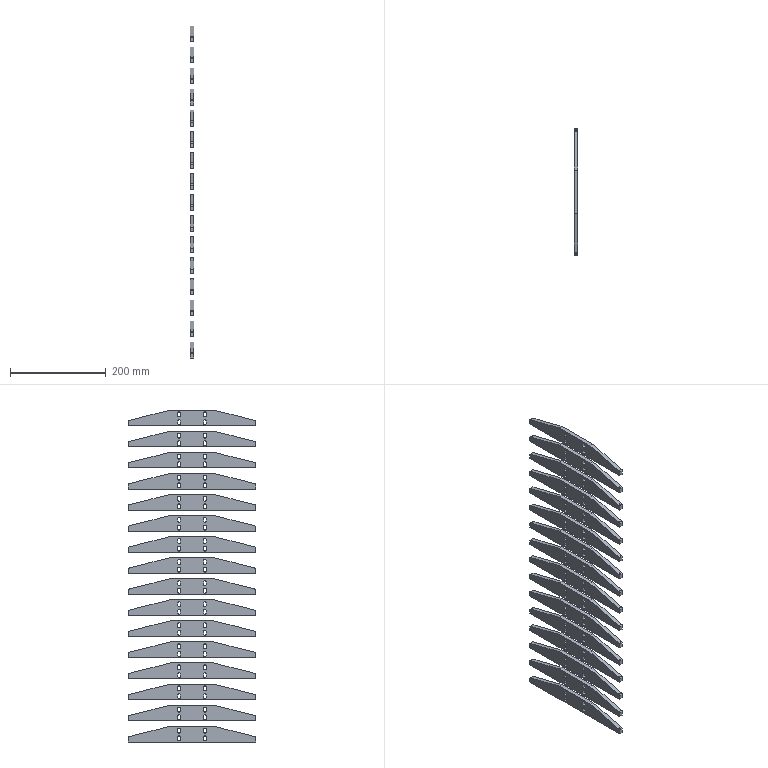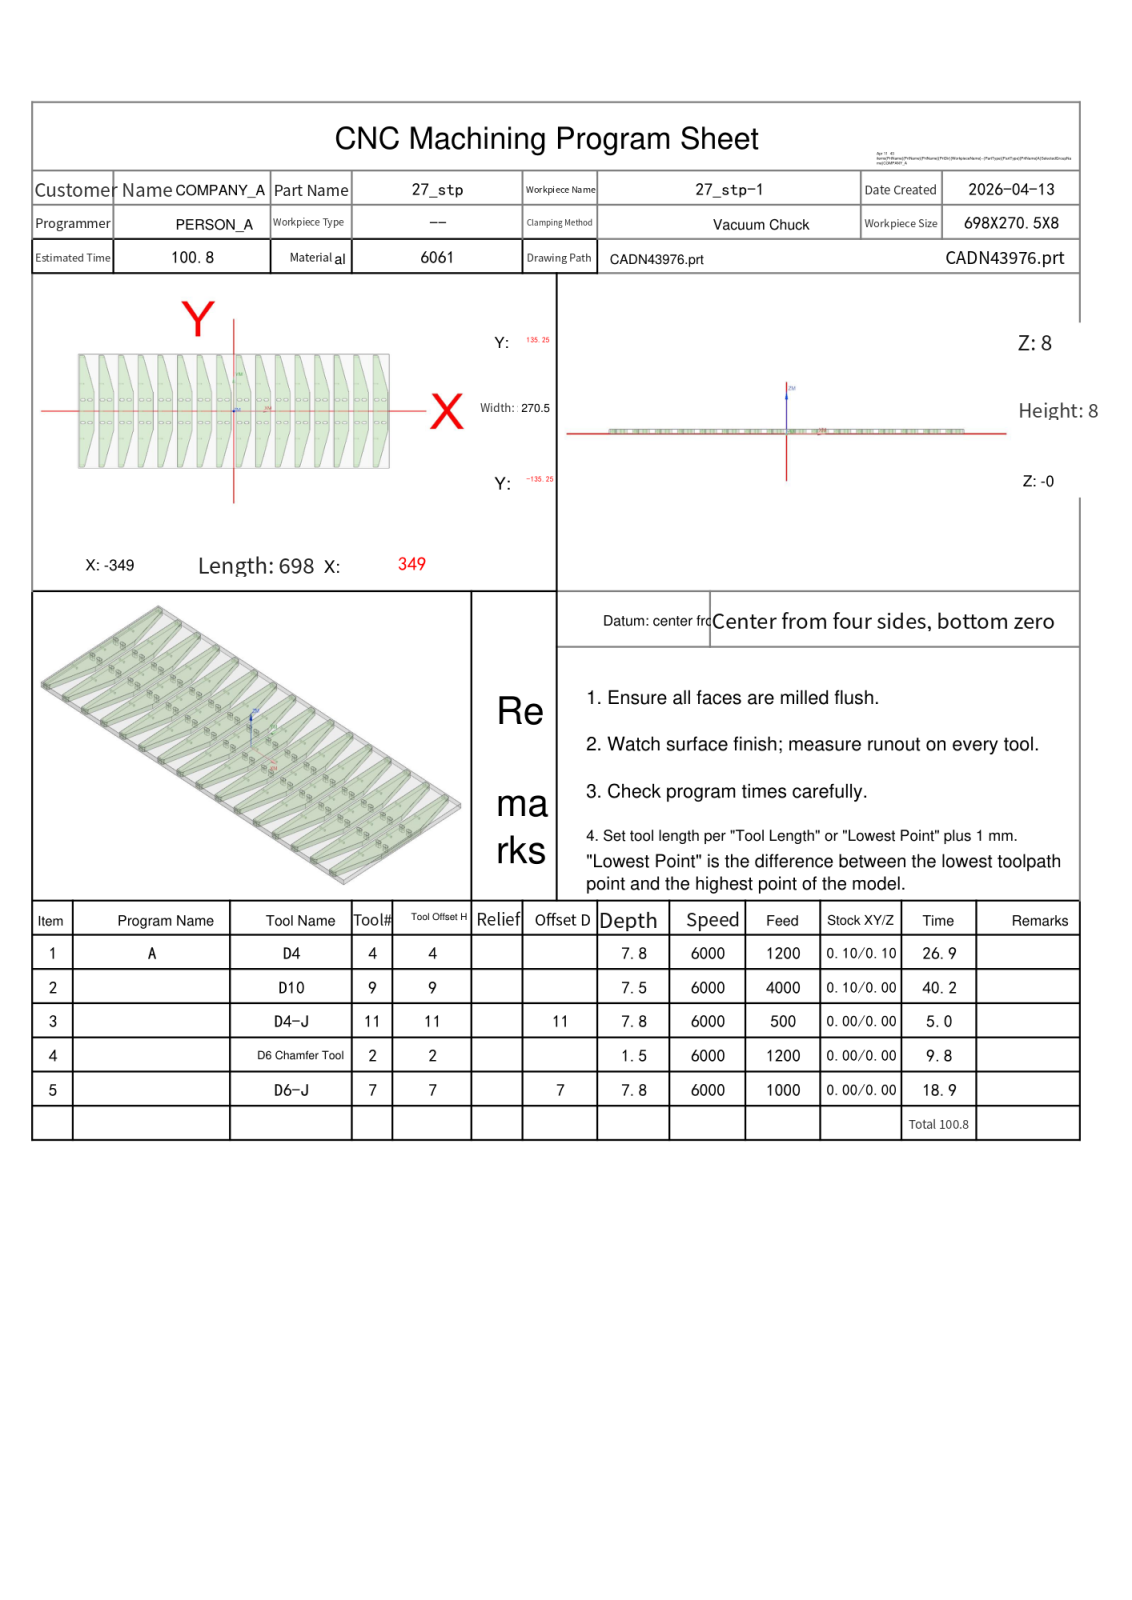NC program | NX | posted by the shop | part box 8 x 265.5 x 693 mm
Lines 19372 to 21683 of 21683, first 1858 of 2312 lines:
N4 T02 M06
(D6 Chamfer Tool  D=6. R=0. H=02 ce=0.00 di=0.00)
G00 G90 G54 X311.372 Y-.25 M03 S6000
G43 H02 Z28.
M08
Z10.099
G01 Z6.5 F1200.
G03 X311.672 Y-.33 I.3 J.52
X312.192 Y-.03 I0.0 J.6
G01 X312.2 Y0.0
Y132.75
G02 X313.5 Y134.05 I1.3 J0.0
G01 X322.012
G02 X326.18 Y130.804 I0.0 J-4.3
G01 X347.76 Y45.484
X347.79 Y45.326
X347.8 Y45.166
Y-45.166
X347.79 Y-45.326
X347.76 Y-45.484
X326.18 Y-130.804
G02 X322.012 Y-134.05 I-4.169 J1.054
G01 X313.5
G02 X312.2 Y-132.75 I0.0 J1.3
G01 Y0.0
X312.192 Y.03
G03 X311.672 Y.33 I-.52 J-.3
X311.372 Y.25 I0.0 J-.6
G01 Z10.099
G00 Z28.
X336.95 Y26.378
Z10.099
G01 Z6.5
G03 X336.87 Y26.078 I.52 J-.3
X337.17 Y25.558 I.6 J0.0
G01 X337.2 Y25.55
X339.7
G03 X341.15 Y27. I0.0 J1.45
X339.7 Y28.45 I-1.45 J0.0
G01 X334.7
G03 X333.25 Y27. I0.0 J-1.45
X334.7 Y25.55 I1.45 J0.0
G01 X337.2
X337.23 Y25.558
G03 X337.53 Y26.078 I-.3 J.52
X337.45 Y26.378 I-.6 J0.0
G01 Z10.099
G00 Z28.
X320.95
Z10.099
G01 Z6.5
G03 X320.87 Y26.078 I.52 J-.3
X321.17 Y25.558 I.6 J0.0
G01 X321.2 Y25.55
X323.7
G03 X325.15 Y27. I0.0 J1.45
X323.7 Y28.45 I-1.45 J0.0
G01 X318.7
G03 X317.25 Y27. I0.0 J-1.45
X318.7 Y25.55 I1.45 J0.0
G01 X321.2
X321.23 Y25.558
G03 X321.53 Y26.078 I-.3 J.52
X321.45 Y26.378 I-.6 J0.0
G01 Z10.099
G00 Z28.
X320.95 Y-27.622
Z10.099
G01 Z6.5
G03 X320.87 Y-27.922 I.52 J-.3
X321.17 Y-28.442 I.6 J0.0
G01 X321.2 Y-28.45
X323.7
G03 X325.15 Y-27. I0.0 J1.45
X323.7 Y-25.55 I-1.45 J0.0
G01 X318.7
G03 X317.25 Y-27. I0.0 J-1.45
X318.7 Y-28.45 I1.45 J0.0
G01 X321.2
X321.23 Y-28.442
G03 X321.53 Y-27.922 I-.3 J.52
X321.45 Y-27.622 I-.6 J0.0
G01 Z10.099
G00 Z28.
X336.95
Z10.099
G01 Z6.5
G03 X336.87 Y-27.922 I.52 J-.3
X337.17 Y-28.442 I.6 J0.0
G01 X337.2 Y-28.45
X339.7
G03 X341.15 Y-27. I0.0 J1.45
X339.7 Y-25.55 I-1.45 J0.0
G01 X334.7
G03 X333.25 Y-27. I0.0 J-1.45
X334.7 Y-28.45 I1.45 J0.0
G01 X337.2
X337.23 Y-28.442
G03 X337.53 Y-27.922 I-.3 J.52
X337.45 Y-27.622 I-.6 J0.0
G01 Z10.099
G00 Z28.
X267.372 Y-.25
Z10.099
G01 Z6.5
G03 X267.672 Y-.33 I.3 J.52
X268.192 Y-.03 I0.0 J.6
G01 X268.2 Y0.0
Y132.75
G02 X269.5 Y134.05 I1.3 J0.0
G01 X278.012
G02 X282.18 Y130.804 I0.0 J-4.3
G01 X303.76 Y45.484
X303.79 Y45.326
X303.8 Y45.166
Y-45.166
X303.79 Y-45.326
X303.76 Y-45.484
X282.18 Y-130.804
G02 X278.012 Y-134.05 I-4.169 J1.054
G01 X269.5
G02 X268.2 Y-132.75 I0.0 J1.3
G01 Y0.0
X268.192 Y.03
G03 X267.672 Y.33 I-.52 J-.3
X267.372 Y.25 I0.0 J-.6
G01 Z10.099
G00 Z28.
X293.45 Y27.622
Z10.099
G01 Z6.5
G03 X293.53 Y27.922 I-.52 J.3
X293.23 Y28.442 I-.6 J0.0
G01 X293.2 Y28.45
X290.7
G03 X289.25 Y27. I0.0 J-1.45
X290.7 Y25.55 I1.45 J0.0
G01 X295.7
G03 X297.15 Y27. I0.0 J1.45
X295.7 Y28.45 I-1.45 J0.0
G01 X293.2
X293.17 Y28.442
G03 X292.87 Y27.922 I.3 J-.52
X292.95 Y27.622 I.6 J0.0
G01 Z10.099
G00 Z28.
X277.45
Z10.099
G01 Z6.5
G03 X277.53 Y27.922 I-.52 J.3
X277.23 Y28.442 I-.6 J0.0
G01 X277.2 Y28.45
X274.7
G03 X273.25 Y27. I0.0 J-1.45
X274.7 Y25.55 I1.45 J0.0
G01 X279.7
G03 X281.15 Y27. I0.0 J1.45
X279.7 Y28.45 I-1.45 J0.0
G01 X277.2
X277.17 Y28.442
G03 X276.87 Y27.922 I.3 J-.52
X276.95 Y27.622 I.6 J0.0
G01 Z10.099
G00 Z28.
X277.45 Y-26.378
Z10.099
G01 Z6.5
G03 X277.53 Y-26.078 I-.52 J.3
X277.23 Y-25.558 I-.6 J0.0
G01 X277.2 Y-25.55
X274.7
G03 X273.25 Y-27. I0.0 J-1.45
X274.7 Y-28.45 I1.45 J0.0
G01 X279.7
G03 X281.15 Y-27. I0.0 J1.45
X279.7 Y-25.55 I-1.45 J0.0
G01 X277.2
X277.17 Y-25.558
G03 X276.87 Y-26.078 I.3 J-.52
X276.95 Y-26.378 I.6 J0.0
G01 Z10.099
G00 Z28.
X292.95 Y-27.622
Z10.099
G01 Z6.5
G03 X292.87 Y-27.922 I.52 J-.3
X293.17 Y-28.442 I.6 J0.0
G01 X293.2 Y-28.45
X295.7
G03 X297.15 Y-27. I0.0 J1.45
X295.7 Y-25.55 I-1.45 J0.0
G01 X290.7
G03 X289.25 Y-27. I0.0 J-1.45
X290.7 Y-28.45 I1.45 J0.0
G01 X293.2
X293.23 Y-28.442
G03 X293.53 Y-27.922 I-.3 J.52
X293.45 Y-27.622 I-.6 J0.0
G01 Z10.099
G00 Z28.
X223.372 Y-.25
Z10.099
G01 Z6.5
G03 X223.672 Y-.33 I.3 J.52
X224.192 Y-.03 I0.0 J.6
G01 X224.2 Y0.0
Y132.75
G02 X225.5 Y134.05 I1.3 J0.0
G01 X234.012
G02 X238.18 Y130.804 I0.0 J-4.3
G01 X259.76 Y45.484
X259.79 Y45.326
X259.8 Y45.166
Y-45.166
X259.79 Y-45.326
X259.76 Y-45.484
X238.18 Y-130.804
G02 X234.012 Y-134.05 I-4.169 J1.054
G01 X225.5
G02 X224.2 Y-132.75 I0.0 J1.3
G01 Y0.0
X224.192 Y.03
G03 X223.672 Y.33 I-.52 J-.3
X223.372 Y.25 I0.0 J-.6
G01 Z10.099
G00 Z28.
X248.95 Y26.378
Z10.099
G01 Z6.5
G03 X248.87 Y26.078 I.52 J-.3
X249.17 Y25.558 I.6 J0.0
G01 X249.2 Y25.55
X251.7
G03 X253.15 Y27. I0.0 J1.45
X251.7 Y28.45 I-1.45 J0.0
G01 X246.7
G03 X245.25 Y27. I0.0 J-1.45
X246.7 Y25.55 I1.45 J0.0
G01 X249.2
X249.23 Y25.558
G03 X249.53 Y26.078 I-.3 J.52
X249.45 Y26.378 I-.6 J0.0
G01 Z10.099
G00 Z28.
X232.95
Z10.099
G01 Z6.5
G03 X232.87 Y26.078 I.52 J-.3
X233.17 Y25.558 I.6 J0.0
G01 X233.2 Y25.55
X235.7
G03 X237.15 Y27. I0.0 J1.45
X235.7 Y28.45 I-1.45 J0.0
G01 X230.7
G03 X229.25 Y27. I0.0 J-1.45
X230.7 Y25.55 I1.45 J0.0
G01 X233.2
X233.23 Y25.558
G03 X233.53 Y26.078 I-.3 J.52
X233.45 Y26.378 I-.6 J0.0
G01 Z10.099
G00 Z28.
Y-26.378
Z10.099
G01 Z6.5
G03 X233.53 Y-26.078 I-.52 J.3
X233.23 Y-25.558 I-.6 J0.0
G01 X233.2 Y-25.55
X230.7
G03 X229.25 Y-27. I0.0 J-1.45
X230.7 Y-28.45 I1.45 J0.0
G01 X235.7
G03 X237.15 Y-27. I0.0 J1.45
X235.7 Y-25.55 I-1.45 J0.0
G01 X233.2
X233.17 Y-25.558
G03 X232.87 Y-26.078 I.3 J-.52
X232.95 Y-26.378 I.6 J0.0
G01 Z10.099
G00 Z28.
X249.45
Z10.099
G01 Z6.5
G03 X249.53 Y-26.078 I-.52 J.3
X249.23 Y-25.558 I-.6 J0.0
G01 X249.2 Y-25.55
X246.7
G03 X245.25 Y-27. I0.0 J-1.45
X246.7 Y-28.45 I1.45 J0.0
G01 X251.7
G03 X253.15 Y-27. I0.0 J1.45
X251.7 Y-25.55 I-1.45 J0.0
G01 X249.2
X249.17 Y-25.558
G03 X248.87 Y-26.078 I.3 J-.52
X248.95 Y-26.378 I.6 J0.0
G01 Z10.099
G00 Z28.
X179.372 Y-.25
Z10.099
G01 Z6.5
G03 X179.672 Y-.33 I.3 J.52
X180.192 Y-.03 I0.0 J.6
G01 X180.2 Y0.0
Y132.75
G02 X181.5 Y134.05 I1.3 J0.0
G01 X190.012
G02 X194.18 Y130.804 I0.0 J-4.3
G01 X215.76 Y45.484
X215.79 Y45.326
X215.8 Y45.166
Y-45.166
X215.79 Y-45.326
X215.76 Y-45.484
X194.18 Y-130.804
G02 X190.012 Y-134.05 I-4.169 J1.054
G01 X181.5
G02 X180.2 Y-132.75 I0.0 J1.3
G01 Y0.0
X180.192 Y.03
G03 X179.672 Y.33 I-.52 J-.3
X179.372 Y.25 I0.0 J-.6
G01 Z10.099
G00 Z28.
X204.95 Y26.378
Z10.099
G01 Z6.5
G03 X204.87 Y26.078 I.52 J-.3
X205.17 Y25.558 I.6 J0.0
G01 X205.2 Y25.55
X207.7
G03 X209.15 Y27. I0.0 J1.45
X207.7 Y28.45 I-1.45 J0.0
G01 X202.7
G03 X201.25 Y27. I0.0 J-1.45
X202.7 Y25.55 I1.45 J0.0
G01 X205.2
X205.23 Y25.558
G03 X205.53 Y26.078 I-.3 J.52
X205.45 Y26.378 I-.6 J0.0
G01 Z10.099
G00 Z28.
X188.95
Z10.099
G01 Z6.5
G03 X188.87 Y26.078 I.52 J-.3
X189.17 Y25.558 I.6 J0.0
G01 X189.2 Y25.55
X191.7
G03 X193.15 Y27. I0.0 J1.45
X191.7 Y28.45 I-1.45 J0.0
G01 X186.7
G03 X185.25 Y27. I0.0 J-1.45
X186.7 Y25.55 I1.45 J0.0
G01 X189.2
X189.23 Y25.558
G03 X189.53 Y26.078 I-.3 J.52
X189.45 Y26.378 I-.6 J0.0
G01 Z10.099
G00 Z28.
Y-26.378
Z10.099
G01 Z6.5
G03 X189.53 Y-26.078 I-.52 J.3
X189.23 Y-25.558 I-.6 J0.0
G01 X189.2 Y-25.55
X186.7
G03 X185.25 Y-27. I0.0 J-1.45
X186.7 Y-28.45 I1.45 J0.0
G01 X191.7
G03 X193.15 Y-27. I0.0 J1.45
X191.7 Y-25.55 I-1.45 J0.0
G01 X189.2
X189.17 Y-25.558
G03 X188.87 Y-26.078 I.3 J-.52
X188.95 Y-26.378 I.6 J0.0
G01 Z10.099
G00 Z28.
X205.45
Z10.099
G01 Z6.5
G03 X205.53 Y-26.078 I-.52 J.3
X205.23 Y-25.558 I-.6 J0.0
G01 X205.2 Y-25.55
X202.7
G03 X201.25 Y-27. I0.0 J-1.45
X202.7 Y-28.45 I1.45 J0.0
G01 X207.7
G03 X209.15 Y-27. I0.0 J1.45
X207.7 Y-25.55 I-1.45 J0.0
G01 X205.2
X205.17 Y-25.558
G03 X204.87 Y-26.078 I.3 J-.52
X204.95 Y-26.378 I.6 J0.0
G01 Z10.099
G00 Z28.
X135.372 Y-.25
Z10.099
G01 Z6.5
G03 X135.672 Y-.33 I.3 J.52
X136.192 Y-.03 I0.0 J.6
G01 X136.2 Y0.0
Y132.75
G02 X137.5 Y134.05 I1.3 J0.0
G01 X146.012
G02 X150.18 Y130.804 I0.0 J-4.3
G01 X171.76 Y45.484
X171.79 Y45.326
X171.8 Y45.166
Y-45.166
X171.79 Y-45.326
X171.76 Y-45.484
X150.18 Y-130.804
G02 X146.012 Y-134.05 I-4.169 J1.054
G01 X137.5
G02 X136.2 Y-132.75 I0.0 J1.3
G01 Y0.0
X136.192 Y.03
G03 X135.672 Y.33 I-.52 J-.3
X135.372 Y.25 I0.0 J-.6
G01 Z10.099
G00 Z28.
X160.95 Y26.378
Z10.099
G01 Z6.5
G03 X160.87 Y26.078 I.52 J-.3
X161.17 Y25.558 I.6 J0.0
G01 X161.2 Y25.55
X163.7
G03 X165.15 Y27. I0.0 J1.45
X163.7 Y28.45 I-1.45 J0.0
G01 X158.7
G03 X157.25 Y27. I0.0 J-1.45
X158.7 Y25.55 I1.45 J0.0
G01 X161.2
X161.23 Y25.558
G03 X161.53 Y26.078 I-.3 J.52
X161.45 Y26.378 I-.6 J0.0
G01 Z10.099
G00 Z28.
X144.95
Z10.099
G01 Z6.5
G03 X144.87 Y26.078 I.52 J-.3
X145.17 Y25.558 I.6 J0.0
G01 X145.2 Y25.55
X147.7
G03 X149.15 Y27. I0.0 J1.45
X147.7 Y28.45 I-1.45 J0.0
G01 X142.7
G03 X141.25 Y27. I0.0 J-1.45
X142.7 Y25.55 I1.45 J0.0
G01 X145.2
X145.23 Y25.558
G03 X145.53 Y26.078 I-.3 J.52
X145.45 Y26.378 I-.6 J0.0
G01 Z10.099
G00 Z28.
Y-26.378
Z10.099
G01 Z6.5
G03 X145.53 Y-26.078 I-.52 J.3
X145.23 Y-25.558 I-.6 J0.0
G01 X145.2 Y-25.55
X142.7
G03 X141.25 Y-27. I0.0 J-1.45
X142.7 Y-28.45 I1.45 J0.0
G01 X147.7
G03 X149.15 Y-27. I0.0 J1.45
X147.7 Y-25.55 I-1.45 J0.0
G01 X145.2
X145.17 Y-25.558
G03 X144.87 Y-26.078 I.3 J-.52
X144.95 Y-26.378 I.6 J0.0
G01 Z10.099
G00 Z28.
X161.45
Z10.099
G01 Z6.5
G03 X161.53 Y-26.078 I-.52 J.3
X161.23 Y-25.558 I-.6 J0.0
G01 X161.2 Y-25.55
X158.7
G03 X157.25 Y-27. I0.0 J-1.45
X158.7 Y-28.45 I1.45 J0.0
G01 X163.7
G03 X165.15 Y-27. I0.0 J1.45
X163.7 Y-25.55 I-1.45 J0.0
G01 X161.2
X161.17 Y-25.558
G03 X160.87 Y-26.078 I.3 J-.52
X160.95 Y-26.378 I.6 J0.0
G01 Z10.099
G00 Z28.
X91.372 Y-.25
Z10.099
G01 Z6.5
G03 X91.672 Y-.33 I.3 J.52
X92.192 Y-.03 I0.0 J.6
G01 X92.2 Y0.0
Y132.75
G02 X93.5 Y134.05 I1.3 J0.0
G01 X102.012
G02 X106.18 Y130.804 I0.0 J-4.3
G01 X127.76 Y45.484
X127.79 Y45.326
X127.8 Y45.166
Y-45.166
X127.79 Y-45.326
X127.76 Y-45.484
X106.18 Y-130.804
G02 X102.012 Y-134.05 I-4.169 J1.054
G01 X93.5
G02 X92.2 Y-132.75 I0.0 J1.3
G01 Y0.0
X92.192 Y.03
G03 X91.672 Y.33 I-.52 J-.3
X91.372 Y.25 I0.0 J-.6
G01 Z10.099
G00 Z28.
X116.95 Y26.378
Z10.099
G01 Z6.5
G03 X116.87 Y26.078 I.52 J-.3
X117.17 Y25.558 I.6 J0.0
G01 X117.2 Y25.55
X119.7
G03 X121.15 Y27. I0.0 J1.45
X119.7 Y28.45 I-1.45 J0.0
G01 X114.7
G03 X113.25 Y27. I0.0 J-1.45
X114.7 Y25.55 I1.45 J0.0
G01 X117.2
X117.23 Y25.558
G03 X117.53 Y26.078 I-.3 J.52
X117.45 Y26.378 I-.6 J0.0
G01 Z10.099
G00 Z28.
X100.95
Z10.099
G01 Z6.5
G03 X100.87 Y26.078 I.52 J-.3
X101.17 Y25.558 I.6 J0.0
G01 X101.2 Y25.55
X103.7
G03 X105.15 Y27. I0.0 J1.45
X103.7 Y28.45 I-1.45 J0.0
G01 X98.7
G03 X97.25 Y27. I0.0 J-1.45
X98.7 Y25.55 I1.45 J0.0
G01 X101.2
X101.23 Y25.558
G03 X101.53 Y26.078 I-.3 J.52
X101.45 Y26.378 I-.6 J0.0
G01 Z10.099
G00 Z28.
Y-26.378
Z10.099
G01 Z6.5
G03 X101.53 Y-26.078 I-.52 J.3
X101.23 Y-25.558 I-.6 J0.0
G01 X101.2 Y-25.55
X98.7
G03 X97.25 Y-27. I0.0 J-1.45
X98.7 Y-28.45 I1.45 J0.0
G01 X103.7
G03 X105.15 Y-27. I0.0 J1.45
X103.7 Y-25.55 I-1.45 J0.0
G01 X101.2
X101.17 Y-25.558
G03 X100.87 Y-26.078 I.3 J-.52
X100.95 Y-26.378 I.6 J0.0
G01 Z10.099
G00 Z28.
X117.45
Z10.099
G01 Z6.5
G03 X117.53 Y-26.078 I-.52 J.3
X117.23 Y-25.558 I-.6 J0.0
G01 X117.2 Y-25.55
X114.7
G03 X113.25 Y-27. I0.0 J-1.45
X114.7 Y-28.45 I1.45 J0.0
G01 X119.7
G03 X121.15 Y-27. I0.0 J1.45
X119.7 Y-25.55 I-1.45 J0.0
G01 X117.2
X117.17 Y-25.558
G03 X116.87 Y-26.078 I.3 J-.52
X116.95 Y-26.378 I.6 J0.0
G01 Z10.099
G00 Z28.
X47.372 Y-.25
Z10.099
G01 Z6.5
G03 X47.672 Y-.33 I.3 J.52
X48.192 Y-.03 I0.0 J.6
G01 X48.2 Y0.0
Y132.75
G02 X49.5 Y134.05 I1.3 J0.0
G01 X58.012
G02 X62.18 Y130.804 I0.0 J-4.3
G01 X83.76 Y45.484
X83.79 Y45.326
X83.8 Y45.166
Y-45.166
X83.79 Y-45.326
X83.76 Y-45.484
X62.18 Y-130.804
G02 X58.012 Y-134.05 I-4.169 J1.054
G01 X49.5
G02 X48.2 Y-132.75 I0.0 J1.3
G01 Y0.0
X48.192 Y.03
G03 X47.672 Y.33 I-.52 J-.3
X47.372 Y.25 I0.0 J-.6
G01 Z10.099
G00 Z28.
X72.95 Y26.378
Z10.099
G01 Z6.5
G03 X72.87 Y26.078 I.52 J-.3
X73.17 Y25.558 I.6 J0.0
G01 X73.2 Y25.55
X75.7
G03 X77.15 Y27. I0.0 J1.45
X75.7 Y28.45 I-1.45 J0.0
G01 X70.7
G03 X69.25 Y27. I0.0 J-1.45
X70.7 Y25.55 I1.45 J0.0
G01 X73.2
X73.23 Y25.558
G03 X73.53 Y26.078 I-.3 J.52
X73.45 Y26.378 I-.6 J0.0
G01 Z10.099
G00 Z28.
X56.95
Z10.099
G01 Z6.5
G03 X56.87 Y26.078 I.52 J-.3
X57.17 Y25.558 I.6 J0.0
G01 X57.2 Y25.55
X59.7
G03 X61.15 Y27. I0.0 J1.45
X59.7 Y28.45 I-1.45 J0.0
G01 X54.7
G03 X53.25 Y27. I0.0 J-1.45
X54.7 Y25.55 I1.45 J0.0
G01 X57.2
X57.23 Y25.558
G03 X57.53 Y26.078 I-.3 J.52
X57.45 Y26.378 I-.6 J0.0
G01 Z10.099
G00 Z28.
Y-26.378
Z10.099
G01 Z6.5
G03 X57.53 Y-26.078 I-.52 J.3
X57.23 Y-25.558 I-.6 J0.0
G01 X57.2 Y-25.55
X54.7
G03 X53.25 Y-27. I0.0 J-1.45
X54.7 Y-28.45 I1.45 J0.0
G01 X59.7
G03 X61.15 Y-27. I0.0 J1.45
X59.7 Y-25.55 I-1.45 J0.0
G01 X57.2
X57.17 Y-25.558
G03 X56.87 Y-26.078 I.3 J-.52
X56.95 Y-26.378 I.6 J0.0
G01 Z10.099
G00 Z28.
X73.45
Z10.099
G01 Z6.5
G03 X73.53 Y-26.078 I-.52 J.3
X73.23 Y-25.558 I-.6 J0.0
G01 X73.2 Y-25.55
X70.7
G03 X69.25 Y-27. I0.0 J-1.45
X70.7 Y-28.45 I1.45 J0.0
G01 X75.7
G03 X77.15 Y-27. I0.0 J1.45
X75.7 Y-25.55 I-1.45 J0.0
G01 X73.2
X73.17 Y-25.558
G03 X72.87 Y-26.078 I.3 J-.52
X72.95 Y-26.378 I.6 J0.0
G01 Z10.099
G00 Z28.
X3.372 Y-.25
Z10.099
G01 Z6.5
G03 X3.672 Y-.33 I.3 J.52
X4.192 Y-.03 I0.0 J.6
G01 X4.2 Y0.0
Y132.75
G02 X5.5 Y134.05 I1.3 J0.0
G01 X14.012
G02 X18.18 Y130.804 I0.0 J-4.3
G01 X39.76 Y45.484
X39.79 Y45.326
X39.8 Y45.166
Y-45.166
X39.79 Y-45.326
X39.76 Y-45.484
X18.18 Y-130.804
G02 X14.012 Y-134.05 I-4.169 J1.054
G01 X5.5
G02 X4.2 Y-132.75 I0.0 J1.3
G01 Y0.0
X4.192 Y.03
G03 X3.672 Y.33 I-.52 J-.3
X3.372 Y.25 I0.0 J-.6
G01 Z10.099
G00 Z28.
X28.95 Y26.378
Z10.099
G01 Z6.5
G03 X28.87 Y26.078 I.52 J-.3
X29.17 Y25.558 I.6 J0.0
G01 X29.2 Y25.55
X31.7
G03 X33.15 Y27. I0.0 J1.45
X31.7 Y28.45 I-1.45 J0.0
G01 X26.7
G03 X25.25 Y27. I0.0 J-1.45
X26.7 Y25.55 I1.45 J0.0
G01 X29.2
X29.23 Y25.558
G03 X29.53 Y26.078 I-.3 J.52
X29.45 Y26.378 I-.6 J0.0
G01 Z10.099
G00 Z28.
X12.95
Z10.099
G01 Z6.5
G03 X12.87 Y26.078 I.52 J-.3
X13.17 Y25.558 I.6 J0.0
G01 X13.2 Y25.55
X15.7
G03 X17.15 Y27. I0.0 J1.45
X15.7 Y28.45 I-1.45 J0.0
G01 X10.7
G03 X9.25 Y27. I0.0 J-1.45
X10.7 Y25.55 I1.45 J0.0
G01 X13.2
X13.23 Y25.558
G03 X13.53 Y26.078 I-.3 J.52
X13.45 Y26.378 I-.6 J0.0
G01 Z10.099
G00 Z28.
Y-26.378
Z10.099
G01 Z6.5
G03 X13.53 Y-26.078 I-.52 J.3
X13.23 Y-25.558 I-.6 J0.0
G01 X13.2 Y-25.55
X10.7
G03 X9.25 Y-27. I0.0 J-1.45
X10.7 Y-28.45 I1.45 J0.0
G01 X15.7
G03 X17.15 Y-27. I0.0 J1.45
X15.7 Y-25.55 I-1.45 J0.0
G01 X13.2
X13.17 Y-25.558
G03 X12.87 Y-26.078 I.3 J-.52
X12.95 Y-26.378 I.6 J0.0
G01 Z10.099
G00 Z28.
X29.45
Z10.099
G01 Z6.5
G03 X29.53 Y-26.078 I-.52 J.3
X29.23 Y-25.558 I-.6 J0.0
G01 X29.2 Y-25.55
X26.7
G03 X25.25 Y-27. I0.0 J-1.45
X26.7 Y-28.45 I1.45 J0.0
G01 X31.7
G03 X33.15 Y-27. I0.0 J1.45
X31.7 Y-25.55 I-1.45 J0.0
G01 X29.2
X29.17 Y-25.558
G03 X28.87 Y-26.078 I.3 J-.52
X28.95 Y-26.378 I.6 J0.0
G01 Z10.099
G00 Z28.
X-40.628 Y-.25
Z10.099
G01 Z6.5
G03 X-40.328 Y-.33 I.3 J.52
X-39.808 Y-.03 I0.0 J.6
G01 X-39.8 Y0.0
Y132.75
G02 X-38.5 Y134.05 I1.3 J0.0
G01 X-29.988
G02 X-25.82 Y130.804 I0.0 J-4.3
G01 X-4.24 Y45.484
X-4.21 Y45.326
X-4.2 Y45.166
Y-45.166
X-4.21 Y-45.326
X-4.24 Y-45.484
X-25.82 Y-130.804
G02 X-29.988 Y-134.05 I-4.169 J1.054
G01 X-38.5
G02 X-39.8 Y-132.75 I0.0 J1.3
G01 Y0.0
X-39.808 Y.03
G03 X-40.328 Y.33 I-.52 J-.3
X-40.628 Y.25 I0.0 J-.6
G01 Z10.099
G00 Z28.
X-15.05 Y26.378
Z10.099
G01 Z6.5
G03 X-15.13 Y26.078 I.52 J-.3
X-14.83 Y25.558 I.6 J0.0
G01 X-14.8 Y25.55
X-12.3
G03 X-10.85 Y27. I0.0 J1.45
X-12.3 Y28.45 I-1.45 J0.0
G01 X-17.3
G03 X-18.75 Y27. I0.0 J-1.45
X-17.3 Y25.55 I1.45 J0.0
G01 X-14.8
X-14.77 Y25.558
G03 X-14.47 Y26.078 I-.3 J.52
X-14.55 Y26.378 I-.6 J0.0
G01 Z10.099
G00 Z28.
X-31.05
Z10.099
G01 Z6.5
G03 X-31.13 Y26.078 I.52 J-.3
X-30.83 Y25.558 I.6 J0.0
G01 X-30.8 Y25.55
X-28.3
G03 X-26.85 Y27. I0.0 J1.45
X-28.3 Y28.45 I-1.45 J0.0
G01 X-33.3
G03 X-34.75 Y27. I0.0 J-1.45
X-33.3 Y25.55 I1.45 J0.0
G01 X-30.8
X-30.77 Y25.558
G03 X-30.47 Y26.078 I-.3 J.52
X-30.55 Y26.378 I-.6 J0.0
G01 Z10.099
G00 Z28.
Y-26.378
Z10.099
G01 Z6.5
G03 X-30.47 Y-26.078 I-.52 J.3
X-30.77 Y-25.558 I-.6 J0.0
G01 X-30.8 Y-25.55
X-33.3
G03 X-34.75 Y-27. I0.0 J-1.45
X-33.3 Y-28.45 I1.45 J0.0
G01 X-28.3
G03 X-26.85 Y-27. I0.0 J1.45
X-28.3 Y-25.55 I-1.45 J0.0
G01 X-30.8
X-30.83 Y-25.558
G03 X-31.13 Y-26.078 I.3 J-.52
X-31.05 Y-26.378 I.6 J0.0
G01 Z10.099
G00 Z28.
X-14.55
Z10.099
G01 Z6.5
G03 X-14.47 Y-26.078 I-.52 J.3
X-14.77 Y-25.558 I-.6 J0.0
G01 X-14.8 Y-25.55
X-17.3
G03 X-18.75 Y-27. I0.0 J-1.45
X-17.3 Y-28.45 I1.45 J0.0
G01 X-12.3
G03 X-10.85 Y-27. I0.0 J1.45
X-12.3 Y-25.55 I-1.45 J0.0
G01 X-14.8
X-14.83 Y-25.558
G03 X-15.13 Y-26.078 I.3 J-.52
X-15.05 Y-26.378 I.6 J0.0
G01 Z10.099
G00 Z28.
X-84.628 Y-.25
Z10.099
G01 Z6.5
G03 X-84.328 Y-.33 I.3 J.52
X-83.808 Y-.03 I0.0 J.6
G01 X-83.8 Y0.0
Y132.75
G02 X-82.5 Y134.05 I1.3 J0.0
G01 X-73.988
G02 X-69.82 Y130.804 I0.0 J-4.3
G01 X-48.24 Y45.484
X-48.21 Y45.326
X-48.2 Y45.166
Y-45.166
X-48.21 Y-45.326
X-48.24 Y-45.484
X-69.82 Y-130.804
G02 X-73.988 Y-134.05 I-4.169 J1.054
G01 X-82.5
G02 X-83.8 Y-132.75 I0.0 J1.3
G01 Y0.0
X-83.808 Y.03
G03 X-84.328 Y.33 I-.52 J-.3
X-84.628 Y.25 I0.0 J-.6
G01 Z10.099
G00 Z28.
X-59.05 Y26.378
Z10.099
G01 Z6.5
G03 X-59.13 Y26.078 I.52 J-.3
X-58.83 Y25.558 I.6 J0.0
G01 X-58.8 Y25.55
X-56.3
G03 X-54.85 Y27. I0.0 J1.45
X-56.3 Y28.45 I-1.45 J0.0
G01 X-61.3
G03 X-62.75 Y27. I0.0 J-1.45
X-61.3 Y25.55 I1.45 J0.0
G01 X-58.8
X-58.77 Y25.558
G03 X-58.47 Y26.078 I-.3 J.52
X-58.55 Y26.378 I-.6 J0.0
G01 Z10.099
G00 Z28.
X-75.05
Z10.099
G01 Z6.5
G03 X-75.13 Y26.078 I.52 J-.3
X-74.83 Y25.558 I.6 J0.0
G01 X-74.8 Y25.55
X-72.3
G03 X-70.85 Y27. I0.0 J1.45
X-72.3 Y28.45 I-1.45 J0.0
G01 X-77.3
G03 X-78.75 Y27. I0.0 J-1.45
X-77.3 Y25.55 I1.45 J0.0
G01 X-74.8
X-74.77 Y25.558
G03 X-74.47 Y26.078 I-.3 J.52
X-74.55 Y26.378 I-.6 J0.0
G01 Z10.099
G00 Z28.
Y-26.378
Z10.099
G01 Z6.5
G03 X-74.47 Y-26.078 I-.52 J.3
X-74.77 Y-25.558 I-.6 J0.0
G01 X-74.8 Y-25.55
X-77.3
G03 X-78.75 Y-27. I0.0 J-1.45
X-77.3 Y-28.45 I1.45 J0.0
G01 X-72.3
G03 X-70.85 Y-27. I0.0 J1.45
X-72.3 Y-25.55 I-1.45 J0.0
G01 X-74.8
X-74.83 Y-25.558
G03 X-75.13 Y-26.078 I.3 J-.52
X-75.05 Y-26.378 I.6 J0.0
G01 Z10.099
G00 Z28.
X-58.55
Z10.099
G01 Z6.5
G03 X-58.47 Y-26.078 I-.52 J.3
X-58.77 Y-25.558 I-.6 J0.0
G01 X-58.8 Y-25.55
X-61.3
G03 X-62.75 Y-27. I0.0 J-1.45
X-61.3 Y-28.45 I1.45 J0.0
G01 X-56.3
G03 X-54.85 Y-27. I0.0 J1.45
X-56.3 Y-25.55 I-1.45 J0.0
G01 X-58.8
X-58.83 Y-25.558
G03 X-59.13 Y-26.078 I.3 J-.52
X-59.05 Y-26.378 I.6 J0.0
G01 Z10.099
G00 Z28.
X-128.628 Y-.25
Z10.099
G01 Z6.5
G03 X-128.328 Y-.33 I.3 J.52
X-127.808 Y-.03 I0.0 J.6
G01 X-127.8 Y0.0
Y132.75
G02 X-126.5 Y134.05 I1.3 J0.0
G01 X-117.988
G02 X-113.82 Y130.804 I0.0 J-4.3
G01 X-92.24 Y45.484
X-92.21 Y45.326
X-92.2 Y45.166
Y-45.166
X-92.21 Y-45.326
X-92.24 Y-45.484
X-113.82 Y-130.804
G02 X-117.988 Y-134.05 I-4.169 J1.054
G01 X-126.5
G02 X-127.8 Y-132.75 I0.0 J1.3
G01 Y0.0
X-127.808 Y.03
G03 X-128.328 Y.33 I-.52 J-.3
X-128.628 Y.25 I0.0 J-.6
G01 Z10.099
G00 Z28.
X-103.05 Y26.378
Z10.099
G01 Z6.5
G03 X-103.13 Y26.078 I.52 J-.3
X-102.83 Y25.558 I.6 J0.0
G01 X-102.8 Y25.55
X-100.3
G03 X-98.85 Y27. I0.0 J1.45
X-100.3 Y28.45 I-1.45 J0.0
G01 X-105.3
G03 X-106.75 Y27. I0.0 J-1.45
X-105.3 Y25.55 I1.45 J0.0
G01 X-102.8
X-102.77 Y25.558
G03 X-102.47 Y26.078 I-.3 J.52
X-102.55 Y26.378 I-.6 J0.0
G01 Z10.099
G00 Z28.
X-118.55 Y27.622
Z10.099
G01 Z6.5
G03 X-118.47 Y27.922 I-.52 J.3
X-118.77 Y28.442 I-.6 J0.0
G01 X-118.8 Y28.45
X-121.3
G03 X-122.75 Y27. I0.0 J-1.45
X-121.3 Y25.55 I1.45 J0.0
G01 X-116.3
G03 X-114.85 Y27. I0.0 J1.45
X-116.3 Y28.45 I-1.45 J0.0
G01 X-118.8
X-118.83 Y28.442
G03 X-119.13 Y27.922 I.3 J-.52
X-119.05 Y27.622 I.6 J0.0
G01 Z10.099
G00 Z28.
X-118.55 Y-26.378
Z10.099
G01 Z6.5
G03 X-118.47 Y-26.078 I-.52 J.3
X-118.77 Y-25.558 I-.6 J0.0
G01 X-118.8 Y-25.55
X-121.3
G03 X-122.75 Y-27. I0.0 J-1.45
X-121.3 Y-28.45 I1.45 J0.0
G01 X-116.3
G03 X-114.85 Y-27. I0.0 J1.45
X-116.3 Y-25.55 I-1.45 J0.0
G01 X-118.8
X-118.83 Y-25.558
G03 X-119.13 Y-26.078 I.3 J-.52
X-119.05 Y-26.378 I.6 J0.0
G01 Z10.099
G00 Z28.
X-103.05 Y-27.622
Z10.099
G01 Z6.5
G03 X-103.13 Y-27.922 I.52 J-.3
X-102.83 Y-28.442 I.6 J0.0
G01 X-102.8 Y-28.45
X-100.3
G03 X-98.85 Y-27. I0.0 J1.45
X-100.3 Y-25.55 I-1.45 J0.0
G01 X-105.3
G03 X-106.75 Y-27. I0.0 J-1.45
X-105.3 Y-28.45 I1.45 J0.0
G01 X-102.8
X-102.77 Y-28.442
G03 X-102.47 Y-27.922 I-.3 J.52
X-102.55 Y-27.622 I-.6 J0.0
G01 Z10.099
G00 Z28.
X-172.628 Y-.25
Z10.099
G01 Z6.5
G03 X-172.328 Y-.33 I.3 J.52
X-171.808 Y-.03 I0.0 J.6
G01 X-171.8 Y0.0
Y132.75
G02 X-170.5 Y134.05 I1.3 J0.0
G01 X-161.988
G02 X-157.82 Y130.804 I0.0 J-4.3
G01 X-136.24 Y45.484
X-136.21 Y45.326
X-136.2 Y45.166
Y-45.166
X-136.21 Y-45.326
X-136.24 Y-45.484
X-157.82 Y-130.804
G02 X-161.988 Y-134.05 I-4.169 J1.054
G01 X-170.5
G02 X-171.8 Y-132.75 I0.0 J1.3
G01 Y0.0
X-171.808 Y.03
G03 X-172.328 Y.33 I-.52 J-.3
X-172.628 Y.25 I0.0 J-.6
G01 Z10.099
G00 Z28.
X-147.05 Y26.378
Z10.099
G01 Z6.5
G03 X-147.13 Y26.078 I.52 J-.3
X-146.83 Y25.558 I.6 J0.0
G01 X-146.8 Y25.55
X-144.3
G03 X-142.85 Y27. I0.0 J1.45
X-144.3 Y28.45 I-1.45 J0.0
G01 X-149.3
G03 X-150.75 Y27. I0.0 J-1.45
X-149.3 Y25.55 I1.45 J0.0
G01 X-146.8
X-146.77 Y25.558
G03 X-146.47 Y26.078 I-.3 J.52
X-146.55 Y26.378 I-.6 J0.0
G01 Z10.099
G00 Z28.
X-162.55 Y27.622
Z10.099
G01 Z6.5
G03 X-162.47 Y27.922 I-.52 J.3
X-162.77 Y28.442 I-.6 J0.0
G01 X-162.8 Y28.45
X-165.3
G03 X-166.75 Y27. I0.0 J-1.45
X-165.3 Y25.55 I1.45 J0.0
G01 X-160.3
G03 X-158.85 Y27. I0.0 J1.45
X-160.3 Y28.45 I-1.45 J0.0
G01 X-162.8
X-162.83 Y28.442
G03 X-163.13 Y27.922 I.3 J-.52
X-163.05 Y27.622 I.6 J0.0
G01 Z10.099
G00 Z28.
X-162.55 Y-26.378
Z10.099
G01 Z6.5
G03 X-162.47 Y-26.078 I-.52 J.3
X-162.77 Y-25.558 I-.6 J0.0
G01 X-162.8 Y-25.55
X-165.3
G03 X-166.75 Y-27. I0.0 J-1.45
X-165.3 Y-28.45 I1.45 J0.0
G01 X-160.3
G03 X-158.85 Y-27. I0.0 J1.45
X-160.3 Y-25.55 I-1.45 J0.0
G01 X-162.8
X-162.83 Y-25.558
G03 X-163.13 Y-26.078 I.3 J-.52
X-163.05 Y-26.378 I.6 J0.0
G01 Z10.099
G00 Z28.
X-147.05 Y-27.622
Z10.099
G01 Z6.5
G03 X-147.13 Y-27.922 I.52 J-.3
X-146.83 Y-28.442 I.6 J0.0
G01 X-146.8 Y-28.45
X-144.3
G03 X-142.85 Y-27. I0.0 J1.45
X-144.3 Y-25.55 I-1.45 J0.0
G01 X-149.3
G03 X-150.75 Y-27. I0.0 J-1.45
X-149.3 Y-28.45 I1.45 J0.0
G01 X-146.8
X-146.77 Y-28.442
G03 X-146.47 Y-27.922 I-.3 J.52
X-146.55 Y-27.622 I-.6 J0.0
G01 Z10.099
G00 Z28.
X-216.628 Y-.25
Z10.099
G01 Z6.5
G03 X-216.328 Y-.33 I.3 J.52
X-215.808 Y-.03 I0.0 J.6
G01 X-215.8 Y0.0
Y132.75
G02 X-214.5 Y134.05 I1.3 J0.0
G01 X-205.988
G02 X-201.82 Y130.804 I0.0 J-4.3
G01 X-180.24 Y45.484
X-180.21 Y45.326
X-180.2 Y45.166
Y-45.166
X-180.21 Y-45.326
X-180.24 Y-45.484
X-201.82 Y-130.804
G02 X-205.988 Y-134.05 I-4.169 J1.054
G01 X-214.5
G02 X-215.8 Y-132.75 I0.0 J1.3
G01 Y0.0
X-215.808 Y.03
G03 X-216.328 Y.33 I-.52 J-.3
X-216.628 Y.25 I0.0 J-.6
G01 Z10.099
G00 Z28.
X-191.05 Y26.378
Z10.099
G01 Z6.5
G03 X-191.13 Y26.078 I.52 J-.3
X-190.83 Y25.558 I.6 J0.0
G01 X-190.8 Y25.55
X-188.3
G03 X-186.85 Y27. I0.0 J1.45
X-188.3 Y28.45 I-1.45 J0.0
G01 X-193.3
G03 X-194.75 Y27. I0.0 J-1.45
X-193.3 Y25.55 I1.45 J0.0
G01 X-190.8
X-190.77 Y25.558
G03 X-190.47 Y26.078 I-.3 J.52
X-190.55 Y26.378 I-.6 J0.0
G01 Z10.099
G00 Z28.
X-206.55 Y27.622
Z10.099
G01 Z6.5
G03 X-206.47 Y27.922 I-.52 J.3
X-206.77 Y28.442 I-.6 J0.0
G01 X-206.8 Y28.45
X-209.3
G03 X-210.75 Y27. I0.0 J-1.45
X-209.3 Y25.55 I1.45 J0.0
G01 X-204.3
G03 X-202.85 Y27. I0.0 J1.45
X-204.3 Y28.45 I-1.45 J0.0
G01 X-206.8
X-206.83 Y28.442
G03 X-207.13 Y27.922 I.3 J-.52
X-207.05 Y27.622 I.6 J0.0
G01 Z10.099
G00 Z28.
X-206.55 Y-26.378
Z10.099
G01 Z6.5
G03 X-206.47 Y-26.078 I-.52 J.3
X-206.77 Y-25.558 I-.6 J0.0
G01 X-206.8 Y-25.55
X-209.3
G03 X-210.75 Y-27. I0.0 J-1.45
X-209.3 Y-28.45 I1.45 J0.0
G01 X-204.3
G03 X-202.85 Y-27. I0.0 J1.45
X-204.3 Y-25.55 I-1.45 J0.0
G01 X-206.8
X-206.83 Y-25.558
G03 X-207.13 Y-26.078 I.3 J-.52
X-207.05 Y-26.378 I.6 J0.0
G01 Z10.099
G00 Z28.
X-191.05 Y-27.622
Z10.099
G01 Z6.5
G03 X-191.13 Y-27.922 I.52 J-.3
X-190.83 Y-28.442 I.6 J0.0
G01 X-190.8 Y-28.45
X-188.3
G03 X-186.85 Y-27. I0.0 J1.45
X-188.3 Y-25.55 I-1.45 J0.0
G01 X-193.3
G03 X-194.75 Y-27. I0.0 J-1.45
X-193.3 Y-28.45 I1.45 J0.0
G01 X-190.8
X-190.77 Y-28.442
G03 X-190.47 Y-27.922 I-.3 J.52
X-190.55 Y-27.622 I-.6 J0.0
G01 Z10.099
G00 Z28.
X-260.628 Y-.25
Z10.099
G01 Z6.5
G03 X-260.328 Y-.33 I.3 J.52
X-259.808 Y-.03 I0.0 J.6
G01 X-259.8 Y0.0
Y132.75
G02 X-258.5 Y134.05 I1.3 J0.0
G01 X-249.988
G02 X-245.82 Y130.804 I0.0 J-4.3
G01 X-224.24 Y45.484
X-224.21 Y45.326
X-224.2 Y45.166
Y-45.166
X-224.21 Y-45.326
X-224.24 Y-45.484
X-245.82 Y-130.804
G02 X-249.988 Y-134.05 I-4.169 J1.054
G01 X-258.5
G02 X-259.8 Y-132.75 I0.0 J1.3
G01 Y0.0
X-259.808 Y.03
G03 X-260.328 Y.33 I-.52 J-.3
X-260.628 Y.25 I0.0 J-.6
G01 Z10.099
G00 Z28.
X-235.05 Y26.378
Z10.099
G01 Z6.5
G03 X-235.13 Y26.078 I.52 J-.3
X-234.83 Y25.558 I.6 J0.0
G01 X-234.8 Y25.55
X-232.3
G03 X-230.85 Y27. I0.0 J1.45
X-232.3 Y28.45 I-1.45 J0.0
G01 X-237.3
G03 X-238.75 Y27. I0.0 J-1.45
X-237.3 Y25.55 I1.45 J0.0
G01 X-234.8
X-234.77 Y25.558
G03 X-234.47 Y26.078 I-.3 J.52
X-234.55 Y26.378 I-.6 J0.0
G01 Z10.099
G00 Z28.
X-250.55 Y27.622
Z10.099
G01 Z6.5
G03 X-250.47 Y27.922 I-.52 J.3
X-250.77 Y28.442 I-.6 J0.0
G01 X-250.8 Y28.45
X-253.3
G03 X-254.75 Y27. I0.0 J-1.45
X-253.3 Y25.55 I1.45 J0.0
G01 X-248.3
G03 X-246.85 Y27. I0.0 J1.45
X-248.3 Y28.45 I-1.45 J0.0
G01 X-250.8
X-250.83 Y28.442
G03 X-251.13 Y27.922 I.3 J-.52
X-251.05 Y27.622 I.6 J0.0
G01 Z10.099
G00 Z28.
X-250.55 Y-26.378
Z10.099
G01 Z6.5
G03 X-250.47 Y-26.078 I-.52 J.3
X-250.77 Y-25.558 I-.6 J0.0
G01 X-250.8 Y-25.55
X-253.3
G03 X-254.75 Y-27. I0.0 J-1.45
X-253.3 Y-28.45 I1.45 J0.0
G01 X-248.3
G03 X-246.85 Y-27. I0.0 J1.45
X-248.3 Y-25.55 I-1.45 J0.0
G01 X-250.8
X-250.83 Y-25.558
G03 X-251.13 Y-26.078 I.3 J-.52
X-251.05 Y-26.378 I.6 J0.0
G01 Z10.099
G00 Z28.
X-235.05 Y-27.622
Z10.099
G01 Z6.5
G03 X-235.13 Y-27.922 I.52 J-.3
X-234.83 Y-28.442 I.6 J0.0
G01 X-234.8 Y-28.45
X-232.3
G03 X-230.85 Y-27. I0.0 J1.45
X-232.3 Y-25.55 I-1.45 J0.0
G01 X-237.3
G03 X-238.75 Y-27. I0.0 J-1.45
X-237.3 Y-28.45 I1.45 J0.0
G01 X-234.8
X-234.77 Y-28.442
G03 X-234.47 Y-27.922 I-.3 J.52
X-234.55 Y-27.622 I-.6 J0.0
G01 Z10.099
G00 Z28.
X-304.628 Y-.25
Z10.099
G01 Z6.5
G03 X-304.328 Y-.33 I.3 J.52
X-303.808 Y-.03 I0.0 J.6
G01 X-303.8 Y0.0
Y132.75
G02 X-302.5 Y134.05 I1.3 J0.0
G01 X-293.988
G02 X-289.82 Y130.804 I0.0 J-4.3
G01 X-268.24 Y45.484
X-268.21 Y45.326
X-268.2 Y45.166
Y-45.166
X-268.21 Y-45.326
X-268.24 Y-45.484
X-289.82 Y-130.804
G02 X-293.988 Y-134.05 I-4.169 J1.054
G01 X-302.5
G02 X-303.8 Y-132.75 I0.0 J1.3
G01 Y0.0
X-303.808 Y.03
G03 X-304.328 Y.33 I-.52 J-.3
X-304.628 Y.25 I0.0 J-.6
G01 Z10.099
G00 Z28.
X-278.55 Y27.622
Z10.099
G01 Z6.5
G03 X-278.47 Y27.922 I-.52 J.3
X-278.77 Y28.442 I-.6 J0.0
G01 X-278.8 Y28.45
X-281.3
G03 X-282.75 Y27. I0.0 J-1.45
X-281.3 Y25.55 I1.45 J0.0
G01 X-276.3
G03 X-274.85 Y27. I0.0 J1.45
X-276.3 Y28.45 I-1.45 J0.0
G01 X-278.8
X-278.83 Y28.442
G03 X-279.13 Y27.922 I.3 J-.52
X-279.05 Y27.622 I.6 J0.0
G01 Z10.099
G00 Z28.
X-294.55
Z10.099
G01 Z6.5
G03 X-294.47 Y27.922 I-.52 J.3
X-294.77 Y28.442 I-.6 J0.0
G01 X-294.8 Y28.45
X-297.3
G03 X-298.75 Y27. I0.0 J-1.45
X-297.3 Y25.55 I1.45 J0.0
G01 X-292.3
G03 X-290.85 Y27. I0.0 J1.45
X-292.3 Y28.45 I-1.45 J0.0
G01 X-294.8
X-294.83 Y28.442
G03 X-295.13 Y27.922 I.3 J-.52
X-295.05 Y27.622 I.6 J0.0
G01 Z10.099
G00 Z28.
X-294.55 Y-26.378
Z10.099
G01 Z6.5
G03 X-294.47 Y-26.078 I-.52 J.3
X-294.77 Y-25.558 I-.6 J0.0
G01 X-294.8 Y-25.55
X-297.3
G03 X-298.75 Y-27. I0.0 J-1.45
X-297.3 Y-28.45 I1.45 J0.0
G01 X-292.3
G03 X-290.85 Y-27. I0.0 J1.45
X-292.3 Y-25.55 I-1.45 J0.0
G01 X-294.8
X-294.83 Y-25.558
G03 X-295.13 Y-26.078 I.3 J-.52
X-295.05 Y-26.378 I.6 J0.0
G01 Z10.099
G00 Z28.
X-279.05 Y-27.622
Z10.099
G01 Z6.5
G03 X-279.13 Y-27.922 I.52 J-.3
X-278.83 Y-28.442 I.6 J0.0
G01 X-278.8 Y-28.45
X-276.3
G03 X-274.85 Y-27. I0.0 J1.45
X-276.3 Y-25.55 I-1.45 J0.0
G01 X-281.3
G03 X-282.75 Y-27. I0.0 J-1.45
X-281.3 Y-28.45 I1.45 J0.0
G01 X-278.8
X-278.77 Y-28.442
G03 X-278.47 Y-27.922 I-.3 J.52
X-278.55 Y-27.622 I-.6 J0.0
G01 Z10.099
G00 Z28.
X-348.628 Y-.25
Z10.099
G01 Z6.5
G03 X-348.328 Y-.33 I.3 J.52
X-347.808 Y-.03 I0.0 J.6
G01 X-347.8 Y0.0
Y132.75
G02 X-346.5 Y134.05 I1.3 J0.0
G01 X-337.988
G02 X-333.82 Y130.804 I0.0 J-4.3
G01 X-312.24 Y45.484
X-312.21 Y45.326
X-312.2 Y45.166
Y-45.166
X-312.21 Y-45.326
X-312.24 Y-45.484
X-333.82 Y-130.804
G02 X-337.988 Y-134.05 I-4.169 J1.054
G01 X-346.5
G02 X-347.8 Y-132.75 I0.0 J1.3
G01 Y0.0
X-347.808 Y.03
G03 X-348.328 Y.33 I-.52 J-.3
X-348.628 Y.25 I0.0 J-.6
G01 Z10.099
G00 Z28.
X-323.05 Y26.378
Z10.099
G01 Z6.5
G03 X-323.13 Y26.078 I.52 J-.3
X-322.83 Y25.558 I.6 J0.0
G01 X-322.8 Y25.55
X-320.3
G03 X-318.85 Y27. I0.0 J1.45
X-320.3 Y28.45 I-1.45 J0.0
G01 X-325.3
G03 X-326.75 Y27. I0.0 J-1.45
X-325.3 Y25.55 I1.45 J0.0
G01 X-322.8
X-322.77 Y25.558
G03 X-322.47 Y26.078 I-.3 J.52
X-322.55 Y26.378 I-.6 J0.0
G01 Z10.099
G00 Z28.
X-338.55 Y27.622
Z10.099
G01 Z6.5
G03 X-338.47 Y27.922 I-.52 J.3
X-338.77 Y28.442 I-.6 J0.0
G01 X-338.8 Y28.45
X-341.3
G03 X-342.75 Y27. I0.0 J-1.45
X-341.3 Y25.55 I1.45 J0.0
G01 X-336.3
G03 X-334.85 Y27. I0.0 J1.45
X-336.3 Y28.45 I-1.45 J0.0
G01 X-338.8
X-338.83 Y28.442
G03 X-339.13 Y27.922 I.3 J-.52
X-339.05 Y27.622 I.6 J0.0
G01 Z10.099
G00 Z28.
X-338.55 Y-26.378
Z10.099
G01 Z6.5
G03 X-338.47 Y-26.078 I-.52 J.3
X-338.77 Y-25.558 I-.6 J0.0
G01 X-338.8 Y-25.55
X-341.3
G03 X-342.75 Y-27. I0.0 J-1.45
X-341.3 Y-28.45 I1.45 J0.0
G01 X-336.3
G03 X-334.85 Y-27. I0.0 J1.45
X-336.3 Y-25.55 I-1.45 J0.0
G01 X-338.8
X-338.83 Y-25.558
G03 X-339.13 Y-26.078 I.3 J-.52
X-339.05 Y-26.378 I.6 J0.0
G01 Z10.099
G00 Z28.
X-323.05 Y-27.622
Z10.099
G01 Z6.5
G03 X-323.13 Y-27.922 I.52 J-.3
X-322.83 Y-28.442 I.6 J0.0
G01 X-322.8 Y-28.45
X-320.3
G03 X-318.85 Y-27. I0.0 J1.45
X-320.3 Y-25.55 I-1.45 J0.0
G01 X-325.3
G03 X-326.75 Y-27. I0.0 J-1.45
X-325.3 Y-28.45 I1.45 J0.0
G01 X-322.8
X-322.77 Y-28.442
G03 X-322.47 Y-27.922 I-.3 J.52
X-322.55 Y-27.622 I-.6 J0.0
G01 Z10.099
G00 Z28.
G91 G28 Z0.0
M05
M09
G91 G28 Z0.0
M01
N5 T07 M06
(D6-J  D=6. R=0. H=07 ce=0.00 di=0.00)
G00 G90 G54 X328.674 Y132.479 M03 S6000
G43 H07 Z28.
M08
Z1.
G01 Z.5 F1000.
G41 D07
X328.484 Y132.416
G03 X327.798 Y131.466 I.314 J-.949
X327.828 Y131.221 I1. J0.0
G01 X349.5 Y45.539
Y-45.539
X327.828 Y-131.221
G02 X322.012 Y-135.75 I-5.817 J1.471
G01 X313.5
G02 X310.5 Y-132.75 I0.0 J3.
G01 Y132.75
G02 X313.5 Y135.75 I3. J0.0
G01 X322.012
G02 X327.828 Y131.221 I0.0 J-6.
G01 X327.951 Y130.737
G03 X328.92 Y129.982 I.969 J.245
X329.166 Y130.012 I0.0 J1.
G01 G40 X329.36 Y130.061
Z1.
G00 Z28.
X284.674 Y132.479
Z1.
G01 Z.5
G41 D07
X284.484 Y132.416
G03 X283.798 Y131.466 I.314 J-.949
X283.828 Y131.221 I1. J0.0
G01 X305.5 Y45.539
Y-45.539
X283.828 Y-131.221
G02 X278.012 Y-135.75 I-5.817 J1.471
G01 X269.5
G02 X266.5 Y-132.75 I0.0 J3.
G01 Y132.75
G02 X269.5 Y135.75 I3. J0.0
G01 X278.012
G02 X283.828 Y131.221 I0.0 J-6.
G01 X283.951 Y130.737
G03 X284.92 Y129.982 I.969 J.245
X285.166 Y130.012 I0.0 J1.
G01 G40 X285.36 Y130.061
Z1.
G00 Z28.
X240.674 Y132.479
Z1.
G01 Z.5
G41 D07
X240.484 Y132.416
G03 X239.798 Y131.466 I.314 J-.949
X239.828 Y131.221 I1. J0.0
G01 X261.5 Y45.539
Y-45.539
X239.828 Y-131.221
G02 X234.012 Y-135.75 I-5.817 J1.471
G01 X225.5
G02 X222.5 Y-132.75 I0.0 J3.
G01 Y132.75
G02 X225.5 Y135.75 I3. J0.0
G01 X234.012
G02 X239.828 Y131.221 I0.0 J-6.
G01 X239.951 Y130.737
G03 X240.92 Y129.982 I.969 J.245
X241.166 Y130.012 I0.0 J1.
G01 G40 X241.36 Y130.061
Z1.
G00 Z28.
X196.674 Y132.479
Z1.
G01 Z.5
G41 D07
X196.484 Y132.416
G03 X195.798 Y131.466 I.314 J-.949
X195.828 Y131.221 I1. J0.0
G01 X217.5 Y45.539
Y-45.539
X195.828 Y-131.221
G02 X190.012 Y-135.75 I-5.817 J1.471
G01 X181.5
G02 X178.5 Y-132.75 I0.0 J3.
G01 Y132.75
G02 X181.5 Y135.75 I3. J0.0
G01 X190.012
G02 X195.828 Y131.221 I0.0 J-6.
G01 X195.951 Y130.737
G03 X196.92 Y129.982 I.969 J.245
X197.166 Y130.012 I0.0 J1.
G01 G40 X197.36 Y130.061
Z1.
G00 Z28.
X152.674 Y132.479
Z1.
G01 Z.5
G41 D07
X152.484 Y132.416
G03 X151.798 Y131.466 I.314 J-.949
X151.828 Y131.221 I1. J0.0
G01 X173.5 Y45.539
Y-45.539
X151.828 Y-131.221
G02 X146.012 Y-135.75 I-5.817 J1.471
G01 X137.5
G02 X134.5 Y-132.75 I0.0 J3.
G01 Y132.75
G02 X137.5 Y135.75 I3. J0.0
G01 X146.012
G02 X151.828 Y131.221 I0.0 J-6.
G01 X151.951 Y130.737
G03 X152.92 Y129.982 I.969 J.245
X153.166 Y130.012 I0.0 J1.
G01 G40 X153.36 Y130.061
Z1.
G00 Z28.
X108.674 Y132.479
Z1.
G01 Z.5
G41 D07
X108.484 Y132.416
G03 X107.798 Y131.466 I.314 J-.949
X107.828 Y131.221 I1. J0.0
G01 X129.5 Y45.539
Y-45.539
X107.828 Y-131.221
G02 X102.012 Y-135.75 I-5.817 J1.471
G01 X93.5
G02 X90.5 Y-132.75 I0.0 J3.
G01 Y132.75
G02 X93.5 Y135.75 I3. J0.0
G01 X102.012
G02 X107.828 Y131.221 I0.0 J-6.
G01 X107.951 Y130.737
G03 X108.92 Y129.982 I.969 J.245
X109.166 Y130.012 I0.0 J1.
G01 G40 X109.36 Y130.061
Z1.
G00 Z28.
X64.674 Y132.479
Z1.
G01 Z.5
G41 D07
X64.484 Y132.416
G03 X63.798 Y131.466 I.314 J-.949
X63.828 Y131.221 I1. J0.0
G01 X85.5 Y45.539
Y-45.539
X63.828 Y-131.221
G02 X58.012 Y-135.75 I-5.817 J1.471
G01 X49.5
G02 X46.5 Y-132.75 I0.0 J3.
G01 Y132.75
G02 X49.5 Y135.75 I3. J0.0
G01 X58.012
G02 X63.828 Y131.221 I0.0 J-6.
G01 X63.951 Y130.737
G03 X64.92 Y129.982 I.969 J.245
X65.166 Y130.012 I0.0 J1.
G01 G40 X65.36 Y130.061
Z1.
G00 Z28.
X20.674 Y132.479
Z1.
G01 Z.5
G41 D07
X20.484 Y132.416
G03 X19.798 Y131.466 I.314 J-.949
X19.828 Y131.221 I1. J0.0
G01 X41.5 Y45.539
Y-45.539
X19.828 Y-131.221
G02 X14.012 Y-135.75 I-5.817 J1.471
G01 X5.5
G02 X2.5 Y-132.75 I0.0 J3.
G01 Y132.75
G02 X5.5 Y135.75 I3. J0.0
G01 X14.012
G02 X19.828 Y131.221 I0.0 J-6.
G01 X19.951 Y130.737
G03 X20.92 Y129.982 I.969 J.245
X21.166 Y130.012 I0.0 J1.
G01 G40 X21.36 Y130.061
Z1.
G00 Z28.
X-23.326 Y132.479
Z1.
G01 Z.5
G41 D07
X-23.516 Y132.416
G03 X-24.202 Y131.466 I.314 J-.949
X-24.172 Y131.221 I1. J0.0
G01 X-2.5 Y45.539
Y-45.539
X-24.172 Y-131.221
G02 X-29.988 Y-135.75 I-5.817 J1.471
G01 X-38.5
G02 X-41.5 Y-132.75 I0.0 J3.
G01 Y132.75
G02 X-38.5 Y135.75 I3. J0.0
G01 X-29.988
G02 X-24.172 Y131.221 I0.0 J-6.
G01 X-24.049 Y130.737
G03 X-23.08 Y129.982 I.969 J.245
X-22.834 Y130.012 I0.0 J1.
G01 G40 X-22.64 Y130.061
Z1.
G00 Z28.
X-67.326 Y132.479
Z1.
G01 Z.5
G41 D07
X-67.516 Y132.416
G03 X-68.202 Y131.466 I.314 J-.949
X-68.172 Y131.221 I1. J0.0
G01 X-46.5 Y45.539
Y-45.539
X-68.172 Y-131.221
G02 X-73.988 Y-135.75 I-5.817 J1.471
G01 X-82.5
G02 X-85.5 Y-132.75 I0.0 J3.
G01 Y132.75
G02 X-82.5 Y135.75 I3. J0.0
G01 X-73.988
G02 X-68.172 Y131.221 I0.0 J-6.
G01 X-68.049 Y130.737
G03 X-67.08 Y129.982 I.969 J.245
X-66.834 Y130.012 I0.0 J1.
G01 G40 X-66.64 Y130.061
Z1.
G00 Z28.
X-111.326 Y132.479
Z1.
G01 Z.5
G41 D07
X-111.516 Y132.416
G03 X-112.202 Y131.466 I.314 J-.949
X-112.172 Y131.221 I1. J0.0
G01 X-90.5 Y45.539
Y-45.539
X-112.172 Y-131.221
G02 X-117.988 Y-135.75 I-5.817 J1.471
G01 X-126.5
G02 X-129.5 Y-132.75 I0.0 J3.
G01 Y132.75
G02 X-126.5 Y135.75 I3. J0.0
G01 X-117.988
G02 X-112.172 Y131.221 I0.0 J-6.
G01 X-112.049 Y130.737
G03 X-111.08 Y129.982 I.969 J.245
X-110.834 Y130.012 I0.0 J1.
G01 G40 X-110.64 Y130.061
Z1.
G00 Z28.
X-155.326 Y132.479
Z1.
G01 Z.5
G41 D07
X-155.516 Y132.416
G03 X-156.202 Y131.466 I.314 J-.949
X-156.172 Y131.221 I1. J0.0
G01 X-134.5 Y45.539
Y-45.539
X-156.172 Y-131.221
G02 X-161.988 Y-135.75 I-5.817 J1.471
G01 X-170.5
G02 X-173.5 Y-132.75 I0.0 J3.
G01 Y132.75
G02 X-170.5 Y135.75 I3. J0.0
G01 X-161.988
G02 X-156.172 Y131.221 I0.0 J-6.
G01 X-156.049 Y130.737
G03 X-155.08 Y129.982 I.969 J.245
X-154.834 Y130.012 I0.0 J1.
G01 G40 X-154.64 Y130.061
Z1.
G00 Z28.
X-199.326 Y132.479